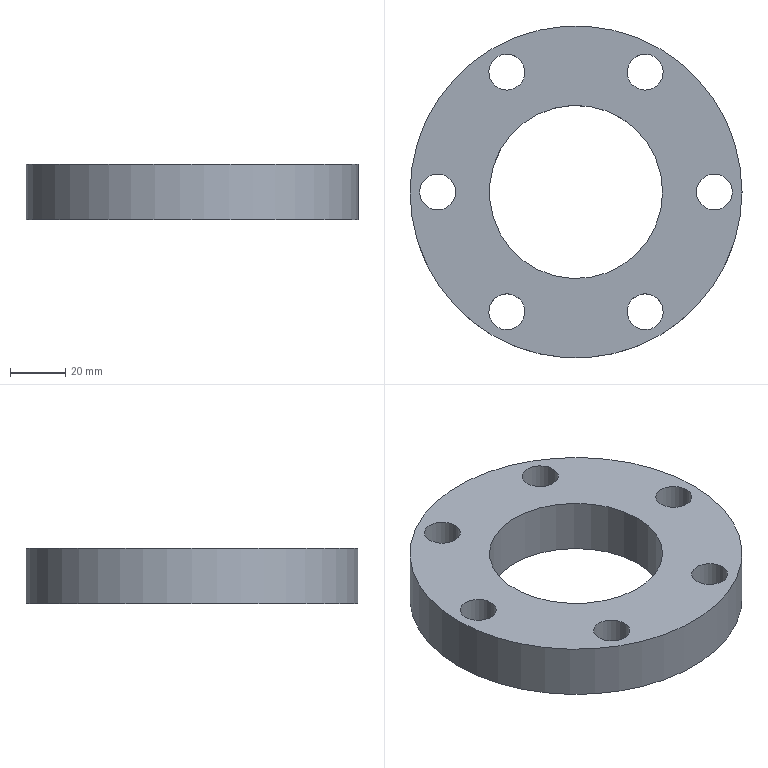Part | NX | 1 solid | 10 faces | box 120 x 120 x 20 mm | volume 148711 mm3 | cylinder 8 | plane 2 | commonest cylinder face diameters 13 x6 62.6 x1 120 x1
STEP:
#1=CARTESIAN_POINT('',(-28.25,-48.93,-20.));
#2=VERTEX_POINT('',#1);
#3=CARTESIAN_POINT('',(-25.,-43.301,-20.));
#4=DIRECTION('',(0.,0.,1.));
#5=DIRECTION('',(-0.5,-0.866,0.));
#6=AXIS2_PLACEMENT_3D('',#3,#4,#5);
#7=CIRCLE('',#6,6.5);
#8=EDGE_CURVE('',#2,#2,#7,.T.);
#9=ORIENTED_EDGE('',*,*,#8,.F.);
#10=EDGE_LOOP('',(#9));
#11=FACE_BOUND('',#10,.T.);
#12=CARTESIAN_POINT('',(-28.25,-48.93,0.));
#13=VERTEX_POINT('',#12);
#14=CARTESIAN_POINT('',(-25.,-43.301,0.));
#15=DIRECTION('',(0.,0.,1.));
#16=DIRECTION('',(-0.5,-0.866,0.));
#17=AXIS2_PLACEMENT_3D('',#14,#15,#16);
#18=CIRCLE('',#17,6.5);
#19=EDGE_CURVE('',#13,#13,#18,.T.);
#20=ORIENTED_EDGE('',*,*,#19,.T.);
#21=EDGE_LOOP('',(#20));
#22=FACE_BOUND('',#21,.T.);
#23=CARTESIAN_POINT('',(-25.,-43.301,-20.));
#24=DIRECTION('',(0.,0.,1.));
#25=DIRECTION('',(1.,0.,0.));
#26=AXIS2_PLACEMENT_3D('',#23,#24,#25);
#27=CYLINDRICAL_SURFACE('',#26,6.5);
#28=ADVANCED_FACE('',(#11,#22),#27,.F.);
#29=CARTESIAN_POINT('',(-28.25,48.93,-20.));
#30=VERTEX_POINT('',#29);
#31=CARTESIAN_POINT('',(-25.,43.301,-20.));
#32=DIRECTION('',(0.,0.,1.));
#33=DIRECTION('',(-0.5,0.866,0.));
#34=AXIS2_PLACEMENT_3D('',#31,#32,#33);
#35=CIRCLE('',#34,6.5);
#36=EDGE_CURVE('',#30,#30,#35,.T.);
#37=ORIENTED_EDGE('',*,*,#36,.F.);
#38=EDGE_LOOP('',(#37));
#39=FACE_BOUND('',#38,.T.);
#40=CARTESIAN_POINT('',(-28.25,48.93,0.));
#41=VERTEX_POINT('',#40);
#42=CARTESIAN_POINT('',(-25.,43.301,0.));
#43=DIRECTION('',(0.,0.,1.));
#44=DIRECTION('',(-0.5,0.866,0.));
#45=AXIS2_PLACEMENT_3D('',#42,#43,#44);
#46=CIRCLE('',#45,6.5);
#47=EDGE_CURVE('',#41,#41,#46,.T.);
#48=ORIENTED_EDGE('',*,*,#47,.T.);
#49=EDGE_LOOP('',(#48));
#50=FACE_BOUND('',#49,.T.);
#51=CARTESIAN_POINT('',(-25.,43.301,-20.));
#52=DIRECTION('',(0.,0.,1.));
#53=DIRECTION('',(1.,0.,0.));
#54=AXIS2_PLACEMENT_3D('',#51,#52,#53);
#55=CYLINDRICAL_SURFACE('',#54,6.5);
#56=ADVANCED_FACE('',(#39,#50),#55,.F.);
#57=CARTESIAN_POINT('',(31.3,0.,-20.));
#58=VERTEX_POINT('',#57);
#59=CARTESIAN_POINT('',(0.,0.,-20.));
#60=DIRECTION('',(0.,0.,1.));
#61=DIRECTION('',(1.,0.,0.));
#62=AXIS2_PLACEMENT_3D('',#59,#60,#61);
#63=CIRCLE('',#62,31.3);
#64=EDGE_CURVE('',#58,#58,#63,.T.);
#65=ORIENTED_EDGE('',*,*,#64,.F.);
#66=EDGE_LOOP('',(#65));
#67=FACE_BOUND('',#66,.T.);
#68=CARTESIAN_POINT('',(31.3,0.,0.));
#69=VERTEX_POINT('',#68);
#70=CARTESIAN_POINT('',(0.,0.,0.));
#71=DIRECTION('',(0.,0.,1.));
#72=DIRECTION('',(1.,0.,0.));
#73=AXIS2_PLACEMENT_3D('',#70,#71,#72);
#74=CIRCLE('',#73,31.3);
#75=EDGE_CURVE('',#69,#69,#74,.T.);
#76=ORIENTED_EDGE('',*,*,#75,.T.);
#77=EDGE_LOOP('',(#76));
#78=FACE_BOUND('',#77,.T.);
#79=CARTESIAN_POINT('',(0.,0.,-20.));
#80=DIRECTION('',(0.,0.,1.));
#81=DIRECTION('',(1.,0.,0.));
#82=AXIS2_PLACEMENT_3D('',#79,#80,#81);
#83=CYLINDRICAL_SURFACE('',#82,31.3);
#84=ADVANCED_FACE('',(#67,#78),#83,.F.);
#85=CARTESIAN_POINT('',(28.25,-48.93,-20.));
#86=VERTEX_POINT('',#85);
#87=CARTESIAN_POINT('',(25.,-43.301,-20.));
#88=DIRECTION('',(0.,0.,1.));
#89=DIRECTION('',(0.5,-0.866,0.));
#90=AXIS2_PLACEMENT_3D('',#87,#88,#89);
#91=CIRCLE('',#90,6.5);
#92=EDGE_CURVE('',#86,#86,#91,.T.);
#93=ORIENTED_EDGE('',*,*,#92,.F.);
#94=EDGE_LOOP('',(#93));
#95=FACE_BOUND('',#94,.T.);
#96=CARTESIAN_POINT('',(28.25,-48.93,0.));
#97=VERTEX_POINT('',#96);
#98=CARTESIAN_POINT('',(25.,-43.301,0.));
#99=DIRECTION('',(0.,0.,1.));
#100=DIRECTION('',(0.5,-0.866,0.));
#101=AXIS2_PLACEMENT_3D('',#98,#99,#100);
#102=CIRCLE('',#101,6.5);
#103=EDGE_CURVE('',#97,#97,#102,.T.);
#104=ORIENTED_EDGE('',*,*,#103,.T.);
#105=EDGE_LOOP('',(#104));
#106=FACE_BOUND('',#105,.T.);
#107=CARTESIAN_POINT('',(25.,-43.301,-20.));
#108=DIRECTION('',(0.,0.,1.));
#109=DIRECTION('',(1.,0.,0.));
#110=AXIS2_PLACEMENT_3D('',#107,#108,#109);
#111=CYLINDRICAL_SURFACE('',#110,6.5);
#112=ADVANCED_FACE('',(#95,#106),#111,.F.);
#113=CARTESIAN_POINT('',(28.25,48.93,-20.));
#114=VERTEX_POINT('',#113);
#115=CARTESIAN_POINT('',(25.,43.301,-20.));
#116=DIRECTION('',(0.,0.,1.));
#117=DIRECTION('',(0.5,0.866,0.));
#118=AXIS2_PLACEMENT_3D('',#115,#116,#117);
#119=CIRCLE('',#118,6.5);
#120=EDGE_CURVE('',#114,#114,#119,.T.);
#121=ORIENTED_EDGE('',*,*,#120,.F.);
#122=EDGE_LOOP('',(#121));
#123=FACE_BOUND('',#122,.T.);
#124=CARTESIAN_POINT('',(28.25,48.93,0.));
#125=VERTEX_POINT('',#124);
#126=CARTESIAN_POINT('',(25.,43.301,0.));
#127=DIRECTION('',(0.,0.,1.));
#128=DIRECTION('',(0.5,0.866,0.));
#129=AXIS2_PLACEMENT_3D('',#126,#127,#128);
#130=CIRCLE('',#129,6.5);
#131=EDGE_CURVE('',#125,#125,#130,.T.);
#132=ORIENTED_EDGE('',*,*,#131,.T.);
#133=EDGE_LOOP('',(#132));
#134=FACE_BOUND('',#133,.T.);
#135=CARTESIAN_POINT('',(25.,43.301,-20.));
#136=DIRECTION('',(0.,0.,1.));
#137=DIRECTION('',(1.,0.,0.));
#138=AXIS2_PLACEMENT_3D('',#135,#136,#137);
#139=CYLINDRICAL_SURFACE('',#138,6.5);
#140=ADVANCED_FACE('',(#123,#134),#139,.F.);
#141=CARTESIAN_POINT('',(56.5,0.,-20.));
#142=VERTEX_POINT('',#141);
#143=CARTESIAN_POINT('',(50.,0.,-20.));
#144=DIRECTION('',(0.,0.,1.));
#145=DIRECTION('',(1.,0.,0.));
#146=AXIS2_PLACEMENT_3D('',#143,#144,#145);
#147=CIRCLE('',#146,6.5);
#148=EDGE_CURVE('',#142,#142,#147,.T.);
#149=ORIENTED_EDGE('',*,*,#148,.F.);
#150=EDGE_LOOP('',(#149));
#151=FACE_BOUND('',#150,.T.);
#152=CARTESIAN_POINT('',(56.5,0.,0.));
#153=VERTEX_POINT('',#152);
#154=CARTESIAN_POINT('',(50.,0.,0.));
#155=DIRECTION('',(0.,0.,1.));
#156=DIRECTION('',(1.,0.,0.));
#157=AXIS2_PLACEMENT_3D('',#154,#155,#156);
#158=CIRCLE('',#157,6.5);
#159=EDGE_CURVE('',#153,#153,#158,.T.);
#160=ORIENTED_EDGE('',*,*,#159,.T.);
#161=EDGE_LOOP('',(#160));
#162=FACE_BOUND('',#161,.T.);
#163=CARTESIAN_POINT('',(50.,0.,-20.));
#164=DIRECTION('',(0.,0.,1.));
#165=DIRECTION('',(1.,0.,0.));
#166=AXIS2_PLACEMENT_3D('',#163,#164,#165);
#167=CYLINDRICAL_SURFACE('',#166,6.5);
#168=ADVANCED_FACE('',(#151,#162),#167,.F.);
#169=CARTESIAN_POINT('',(60.,0.,-20.));
#170=VERTEX_POINT('',#169);
#171=CARTESIAN_POINT('',(0.,0.,-20.));
#172=DIRECTION('',(0.,0.,1.));
#173=DIRECTION('',(1.,0.,0.));
#174=AXIS2_PLACEMENT_3D('',#171,#172,#173);
#175=CIRCLE('',#174,60.);
#176=EDGE_CURVE('',#170,#170,#175,.T.);
#177=ORIENTED_EDGE('',*,*,#176,.T.);
#178=EDGE_LOOP('',(#177));
#179=FACE_BOUND('',#178,.T.);
#180=CARTESIAN_POINT('',(60.,0.,0.));
#181=VERTEX_POINT('',#180);
#182=CARTESIAN_POINT('',(0.,0.,0.));
#183=DIRECTION('',(0.,0.,1.));
#184=DIRECTION('',(1.,0.,0.));
#185=AXIS2_PLACEMENT_3D('',#182,#183,#184);
#186=CIRCLE('',#185,60.);
#187=EDGE_CURVE('',#181,#181,#186,.T.);
#188=ORIENTED_EDGE('',*,*,#187,.F.);
#189=EDGE_LOOP('',(#188));
#190=FACE_BOUND('',#189,.T.);
#191=CARTESIAN_POINT('',(0.,0.,-20.));
#192=DIRECTION('',(0.,0.,1.));
#193=DIRECTION('',(1.,0.,0.));
#194=AXIS2_PLACEMENT_3D('',#191,#192,#193);
#195=CYLINDRICAL_SURFACE('',#194,60.);
#196=ADVANCED_FACE('',(#179,#190),#195,.T.);
#197=CARTESIAN_POINT('',(-56.5,0.,-20.));
#198=VERTEX_POINT('',#197);
#199=CARTESIAN_POINT('',(-50.,0.,-20.));
#200=DIRECTION('',(0.,0.,1.));
#201=DIRECTION('',(-1.,0.,0.));
#202=AXIS2_PLACEMENT_3D('',#199,#200,#201);
#203=CIRCLE('',#202,6.5);
#204=EDGE_CURVE('',#198,#198,#203,.T.);
#205=ORIENTED_EDGE('',*,*,#204,.F.);
#206=EDGE_LOOP('',(#205));
#207=FACE_BOUND('',#206,.T.);
#208=CARTESIAN_POINT('',(-56.5,0.,0.));
#209=VERTEX_POINT('',#208);
#210=CARTESIAN_POINT('',(-50.,0.,0.));
#211=DIRECTION('',(0.,0.,1.));
#212=DIRECTION('',(-1.,0.,0.));
#213=AXIS2_PLACEMENT_3D('',#210,#211,#212);
#214=CIRCLE('',#213,6.5);
#215=EDGE_CURVE('',#209,#209,#214,.T.);
#216=ORIENTED_EDGE('',*,*,#215,.T.);
#217=EDGE_LOOP('',(#216));
#218=FACE_BOUND('',#217,.T.);
#219=CARTESIAN_POINT('',(-50.,0.,-20.));
#220=DIRECTION('',(0.,0.,1.));
#221=DIRECTION('',(1.,0.,0.));
#222=AXIS2_PLACEMENT_3D('',#219,#220,#221);
#223=CYLINDRICAL_SURFACE('',#222,6.5);
#224=ADVANCED_FACE('',(#207,#218),#223,.F.);
#225=ORIENTED_EDGE('',*,*,#176,.F.);
#226=EDGE_LOOP('',(#225));
#227=FACE_BOUND('',#226,.T.);
#228=ORIENTED_EDGE('',*,*,#148,.T.);
#229=EDGE_LOOP('',(#228));
#230=FACE_BOUND('',#229,.T.);
#231=ORIENTED_EDGE('',*,*,#120,.T.);
#232=EDGE_LOOP('',(#231));
#233=FACE_BOUND('',#232,.T.);
#234=ORIENTED_EDGE('',*,*,#92,.T.);
#235=EDGE_LOOP('',(#234));
#236=FACE_BOUND('',#235,.T.);
#237=ORIENTED_EDGE('',*,*,#64,.T.);
#238=EDGE_LOOP('',(#237));
#239=FACE_BOUND('',#238,.T.);
#240=ORIENTED_EDGE('',*,*,#36,.T.);
#241=EDGE_LOOP('',(#240));
#242=FACE_BOUND('',#241,.T.);
#243=ORIENTED_EDGE('',*,*,#8,.T.);
#244=EDGE_LOOP('',(#243));
#245=FACE_BOUND('',#244,.T.);
#246=ORIENTED_EDGE('',*,*,#204,.T.);
#247=EDGE_LOOP('',(#246));
#248=FACE_BOUND('',#247,.T.);
#249=CARTESIAN_POINT('',(25.,0.,-20.));
#250=DIRECTION('',(0.,0.,1.));
#251=DIRECTION('',(1.,0.,0.));
#252=AXIS2_PLACEMENT_3D('',#249,#250,#251);
#253=PLANE('',#252);
#254=ADVANCED_FACE('',(#227,#230,#233,#236,#239,#242,#245,#248),#253,.F.);
#255=ORIENTED_EDGE('',*,*,#187,.T.);
#256=EDGE_LOOP('',(#255));
#257=FACE_BOUND('',#256,.T.);
#258=ORIENTED_EDGE('',*,*,#159,.F.);
#259=EDGE_LOOP('',(#258));
#260=FACE_BOUND('',#259,.T.);
#261=ORIENTED_EDGE('',*,*,#131,.F.);
#262=EDGE_LOOP('',(#261));
#263=FACE_BOUND('',#262,.T.);
#264=ORIENTED_EDGE('',*,*,#103,.F.);
#265=EDGE_LOOP('',(#264));
#266=FACE_BOUND('',#265,.T.);
#267=ORIENTED_EDGE('',*,*,#75,.F.);
#268=EDGE_LOOP('',(#267));
#269=FACE_BOUND('',#268,.T.);
#270=ORIENTED_EDGE('',*,*,#47,.F.);
#271=EDGE_LOOP('',(#270));
#272=FACE_BOUND('',#271,.T.);
#273=ORIENTED_EDGE('',*,*,#19,.F.);
#274=EDGE_LOOP('',(#273));
#275=FACE_BOUND('',#274,.T.);
#276=ORIENTED_EDGE('',*,*,#215,.F.);
#277=EDGE_LOOP('',(#276));
#278=FACE_BOUND('',#277,.T.);
#279=CARTESIAN_POINT('',(25.,0.,0.));
#280=DIRECTION('',(0.,0.,1.));
#281=DIRECTION('',(1.,0.,0.));
#282=AXIS2_PLACEMENT_3D('',#279,#280,#281);
#283=PLANE('',#282);
#284=ADVANCED_FACE('',(#257,#260,#263,#266,#269,#272,#275,#278),#283,.T.);
#285=CLOSED_SHELL('',(#28,#56,#84,#112,#140,#168,#196,#224,#254,#284));
#286=MANIFOLD_SOLID_BREP('',#285);
#287=(LENGTH_UNIT()NAMED_UNIT(*)SI_UNIT(.MILLI.,.METRE.));
#288=UNCERTAINTY_MEASURE_WITH_UNIT(LENGTH_MEASURE(0.00001),#287,'','');
#289=(NAMED_UNIT(*)PLANE_ANGLE_UNIT()SI_UNIT($,.RADIAN.));
#290=(NAMED_UNIT(*)SI_UNIT($,.STERADIAN.)SOLID_ANGLE_UNIT());
#291=(GEOMETRIC_REPRESENTATION_CONTEXT(3)GLOBAL_UNCERTAINTY_ASSIGNED_CONTEXT((#288))GLOBAL_UNIT_ASSIGNED_CONTEXT((#287,#289,#290))REPRESENTATION_CONTEXT('',''));
#292=ADVANCED_BREP_SHAPE_REPRESENTATION('',(#286),#291);